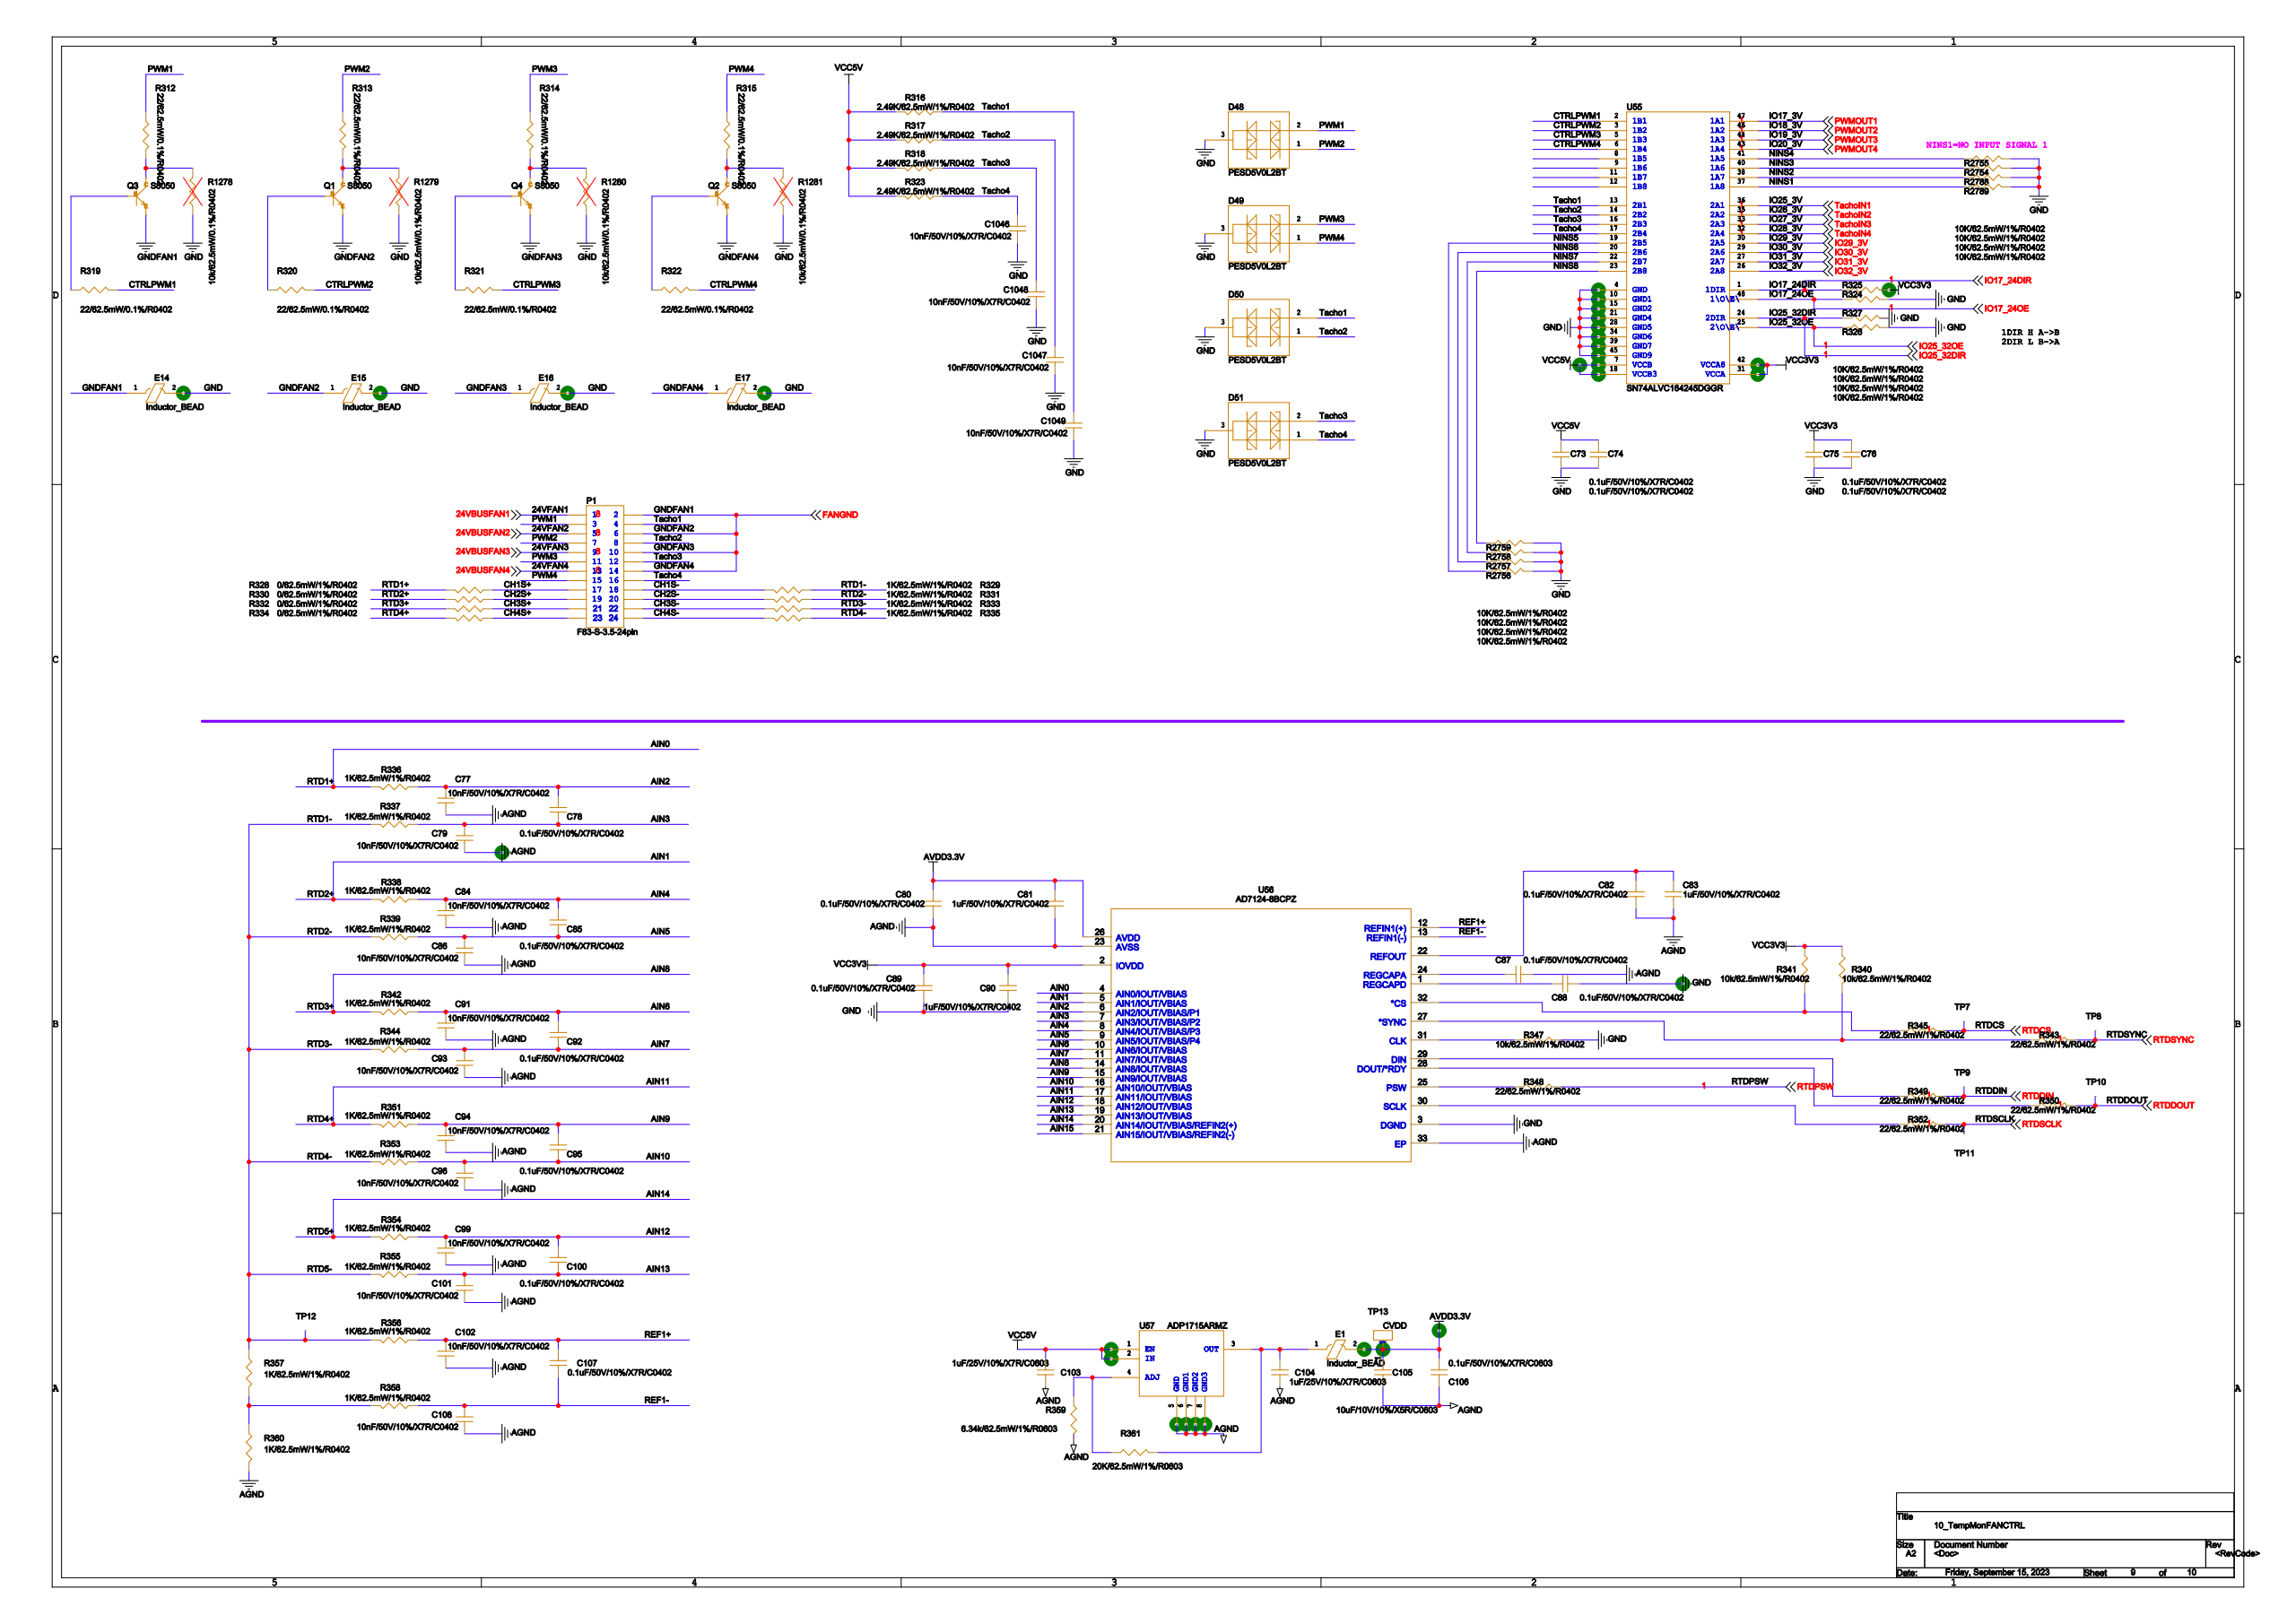Circuit board | Cadence Allegro | 634 parts | 645 nets | one sheet of the schematic
Parts on this sheet (reference | value | footprint):
C73 | 0.1uF/50V/10%/X7R/C0402 | 0402
C74 | 0.1uF/50V/10%/X7R/C0402 | 0402
C75 | 0.1uF/50V/10%/X7R/C0402 | 0402
C76 | 0.1uF/50V/10%/X7R/C0402 | 0402
C77 | 10nF/50V/10%/X7R/C0402 | 0402
C78 | 0.1uF/50V/10%/X7R/C0402 | 0402
C79 | 10nF/50V/10%/X7R/C0402 | 0402
C80 | 0.1uF/50V/10%/X7R/C0402 | 0402
C81 | 1uF/50V/10%/X7R/C0402 | 0402
C82 | 0.1uF/50V/10%/X7R/C0402 | 0402
C83 | 1uF/50V/10%/X7R/C0402 | 0402
C84 | 10nF/50V/10%/X7R/C0402 | 0402
C85 | 0.1uF/50V/10%/X7R/C0402 | 0402
C86 | 10nF/50V/10%/X7R/C0402 | 0402
C87 | 0.1uF/50V/10%/X7R/C0402 | 0402
C88 | 0.1uF/50V/10%/X7R/C0402 | 0402
C89 | 0.1uF/50V/10%/X7R/C0402 | 0402
C90 | 1uF/50V/10%/X7R/C0402 | 0402
C91 | 10nF/50V/10%/X7R/C0402 | 0402
C92 | 0.1uF/50V/10%/X7R/C0402 | 0402
C93 | 10nF/50V/10%/X7R/C0402 | 0402
C94 | 10nF/50V/10%/X7R/C0402 | 0402
C95 | 0.1uF/50V/10%/X7R/C0402 | 0402
C96 | 10nF/50V/10%/X7R/C0402 | 0402
C99 | 10nF/50V/10%/X7R/C0402 | 0402
C100 | 0.1uF/50V/10%/X7R/C0402 | 0402
C101 | 10nF/50V/10%/X7R/C0402 | 0402
C102 | 10nF/50V/10%/X7R/C0402 | 0402
C103 | 1uF/25V/10%/X7R/C0603 | 0603C
C104 | 1uF/25V/10%/X7R/C0603 | 0603C
C105 | 10uF/10V/10%/X5R/C0603 | 0603C
C106 | 0.1uF/50V/10%/X7R/C0603 | 0603C
C107 | 0.1uF/50V/10%/X7R/C0402 | 0402
C108 | 10nF/50V/10%/X7R/C0402 | 0402
C1046 | 10nF/50V/10%/X7R/C0402 | 0402
C1047 | 10nF/50V/10%/X7R/C0402 | 0402
C1048 | 10nF/50V/10%/X7R/C0402 | 0402
C1049 | 10nF/50V/10%/X7R/C0402 | 0402
D48 | PESD5V0L2BT | SOT23
D49 | PESD5V0L2BT | SOT23
D50 | PESD5V0L2BT | SOT23
D51 | PESD5V0L2BT | SOT23
E1 | Inductor_BEAD | 0603R
E14 | Inductor_BEAD | 0603R
E15 | Inductor_BEAD | 0603R
E16 | Inductor_BEAD | 0603R
E17 | Inductor_BEAD | 0603R
P1 | F83-S-3.5-24pin | F83-S-3_5-24PIN
Q1 | S8050 | SOT-23
Q2 | S8050 | SOT-23
Q3 | S8050 | SOT-23
Q4 | S8050 | SOT-23
R312 | 22/62.5mW/0.1%/R0402 | 0402
R313 | 22/62.5mW/0.1%/R0402 | 0402
R314 | 22/62.5mW/0.1%/R0402 | 0402
R315 | 22/62.5mW/0.1%/R0402 | 0402
R316 | 2.49k/62.5mW/1%/R0402 | 0402
R317 | 2.49k/62.5mW/1%/R0402 | 0402
R318 | 2.49k/62.5mW/1%/R0402 | 0402
R319 | 22/62.5mW/0.1%/R0402 | 0402
R320 | 22/62.5mW/0.1%/R0402 | 0402
R321 | 22/62.5mW/0.1%/R0402 | 0402
R322 | 22/62.5mW/0.1%/R0402 | 0402
R323 | 2.49k/62.5mW/1%/R0402 | 0402
R324 | 10K/62.5mW/1%/R0402 | 0402
R325 | 10K/62.5mW/1%/R0402 | 0402
R326 | 10K/62.5mW/1%/R0402 | 0402
R327 | 10K/62.5mW/1%/R0402 | 0402
R328 | 0/62.5mW/1%/R0402 | 0402
R329 | 1K/62.5mW/1%/R0402 | 0402
R330 | 0/62.5mW/1%/R0402 | 0402
R331 | 1K/62.5mW/1%/R0402 | 0402
R332 | 0/62.5mW/1%/R0402 | 0402
R333 | 1K/62.5mW/1%/R0402 | 0402
R334 | 0/62.5mW/1%/R0402 | 0402
R335 | 1K/62.5mW/1%/R0402 | 0402
R336 | 1K/62.5mW/1%/R0402 | 0402
R337 | 1K/62.5mW/1%/R0402 | 0402
R338 | 1K/62.5mW/1%/R0402 | 0402
R339 | 1K/62.5mW/1%/R0402 | 0402
R340 | 10k/62.5mW/1%/R0402 | 0402
R341 | 10k/62.5mW/1%/R0402 | 0402
R342 | 1K/62.5mW/1%/R0402 | 0402
R343 | 22/62.5mW/1%/R0402 | 0402
R344 | 1K/62.5mW/1%/R0402 | 0402
R345 | 22/62.5mW/1%/R0402 | 0402
R347 | 10k/62.5mW/1%/R0402 | 0402
R348 | 22/62.5mW/1%/R0402 | 0402
R349 | 22/62.5mW/1%/R0402 | 0402
R350 | 22/62.5mW/1%/R0402 | 0402
R351 | 1K/62.5mW/1%/R0402 | 0402
R352 | 22/62.5mW/1%/R0402 | 0402
R353 | 1K/62.5mW/1%/R0402 | 0402
R354 | 1K/62.5mW/1%/R0402 | 0402
R355 | 1K/62.5mW/1%/R0402 | 0402
R356 | 1K/62.5mW/1%/R0402 | 0402
R357 | 1K/62.5mW/1%/R0402 | 0402
R358 | 1K/62.5mW/1%/R0402 | 0402
R359 | 6.34k/62.5mW/1%/R0603 | 0603R
R360 | 1K/62.5mW/1%/R0402 | 0402
R361 | 20K/62.5mW/1%/R0603 | 0603R
R1278 | 10k/62.5mW/0.1%/R0402 | 0402
R1279 | 10k/62.5mW/0.1%/R0402 | 0402
R1280 | 10k/62.5mW/0.1%/R0402 | 0402
R1281 | 10k/62.5mW/0.1%/R0402 | 0402
R2754 | 10K/62.5mW/1%/R0402 | 0402
R2755 | 10K/62.5mW/1%/R0402 | 0402
R2756 | 10K/62.5mW/1%/R0402 | 0402
R2757 | 10K/62.5mW/1%/R0402 | 0402
R2758 | 10K/62.5mW/1%/R0402 | 0402
R2759 | 10K/62.5mW/1%/R0402 | 0402
R2788 | 10K/62.5mW/1%/R0402 | 0402
R2789 | 10K/62.5mW/1%/R0402 | 0402
TP7 | TEST POINT A | TEST_12MM
TP8 | TEST POINT A | TEST_12MM
TP9 | TEST POINT A | TEST_12MM
TP10 | TEST POINT A | TEST_12MM
TP11 | TEST POINT A | TEST_12MM
TP12 | TEST POINT A | TEST_12MM
TP13 | CVDD | D0_6
U55 | SN74ALVC164245DGGR | TSSOP-48
U56 | Value | CP_32_12_ADI
U57 | ADP1715ARMZ | MSOP8
Nets of these parts (net: part-pin ...):
AGND: C73-1 C74-1 C75-1 C76-1 C77-2 C79-2 C80-2 C81-2 C82-2 C83-2 C84-2 C86-2 C87-2 C88-2 C89-2 C90-2 C91-2 C93-2 C94-2 C96-2 C99-2 C101-2 C102-2 C103-2 C104-2 C105-2 C106-2 C108-2 C1046-2 C1047-2 C1048-2 C1049-2 D48-3 D49-3 D50-3 D51-3 E14-2 E15-2 E16-2 E17-2 R324-1 R326-1 R327-1 R347-2 R359-1 R360-2 R1278-1 R1279-1 R1280-1 R1281-1 R2754-1 R2755-1 R2756-1 R2757-1 R2758-1 R2759-1 R2788-1 R2789-1 U57-5 U57-6 U57-7 U57-8 U55-4 U55-10 U55-15 U55-21 U55-28 U55-34 U55-39 U55-45 U56-3 U56-23 U56-33
IO25_32DIR: R327-2 U55-24
IO25_32OE: R326-2 U55-25
PWMOUT1: U55-47
3.3V: C75-2 C76-2 C89-1 C90-1 R325-1 R340-1 R341-1 U55-31 U55-42 U56-2
PWMOUT2: U55-46
PWMOUT3: U55-44
PWMOUT4: U55-43
IO17_24DIR: R325-2 U55-1
IO17_24OE: R324-2 U55-48
RTDPSW: R348-2
RTDSYNC: R343-2 TP8-1
RTDDOUT: R350-2 TP10-1
RTDDIN: R349-2 TP9-1
RTDSCLK: R352-2 TP11-1
RTDCS: R345-2 TP7-1
VCC5V: C73-2 C74-2 C103-1 R316-2 R317-2 R318-2 R323-2 U57-1 U57-2 U55-7 U55-18
N23420107: Q3-3 R312-2 R1278-2
N23420396: Q1-3 R313-2 R1279-2
N23420476: Q4-3 R314-2 R1280-2
N23420600: Q2-3 R315-2 R1281-2
TACHO1: C1049-1 D50-2 R316-1 P1-4 U55-13
TACHO2: C1047-1 D50-1 R317-1 P1-8 U55-14
TACHO3: C1048-1 D51-2 R318-1 P1-12 U55-16
TACHO4: C1046-1 D51-1 R323-1 P1-16 U55-17
24VBUSFAN1: P1-1
24VBUSFAN2: P1-5
24VBUSFAN3: P1-9
24VBUSFAN4: P1-13
PWM1: D48-2 R312-1 P1-3
PWM2: D48-1 R313-1 P1-7
PWM3: D49-2 R314-1 P1-11
PWM4: D49-1 R315-1 P1-15
N23420104: Q3-1 R319-1
CTRLPWM1: R319-2 U55-2
N23420393: Q1-1 R320-1
CTRLPWM2: R320-2 U55-3
N23420473: Q4-1 R321-1
CTRLPWM3: R321-2 U55-5
N23420597: Q2-1 R322-1
CTRLPWM4: R322-2 U55-6
AVDD3.3V: C80-1 C81-1 C105-1 C106-1 E1-2 TP13-1 U56-26
N23528814: C104-1 E1-1 R361-1 U57-3
N23528786: R359-2 R361-2 U57-4
FANGND: E14-1 E15-1 E16-1 E17-1 Q1-2 Q2-2 Q3-2 Q4-2 P1-2 P1-6 P1-10 P1-14
CH1S+: R328-1 P1-17
CH1S-: R329-2 P1-18
CH2S+: R330-1 P1-19
CH2S-: R331-2 P1-20
CH3S+: R332-1 P1-21
CH3S-: R333-2 P1-22
CH4S+: R334-1 P1-23
CH4S-: R335-2 P1-24
AIN12: C99-1 C100-1 R354-1 U56-18
AIN13: C100-2 C101-1 R355-1 U56-19
REF1+: C102-1 C107-1 R356-1 U56-12
REF1-: C107-2 C108-1 R358-1 U56-13
N23186180: C87-1 U56-24
AIN6: C91-1 C92-1 R342-1 U56-10
AIN7: C92-2 C93-1 R344-1 U56-11
AIN2: C77-1 C78-1 R336-1 U56-6
AIN3: C78-2 C79-1 R337-1 U56-7
N23186471: C82-1 C83-1 U56-22
AIN4: C84-1 C85-1 R338-1 U56-8
AIN5: C85-2 C86-1 R339-1 U56-9
N23186182: C88-1 U56-1
AIN9: C94-1 C95-1 R351-1 U56-15
AIN10: C95-2 C96-1 R353-1 U56-16
RTD1-: R329-1 R331-1 R333-1 R335-1 R337-2 R339-2 R344-2 R353-2 R355-2 R356-2 R357-1 TP12-1
AIN0: R328-2 R336-2 U56-4
AIN1: R330-2 R338-2 U56-5
AIN8: R332-2 R342-2 U56-14
AIN11: R334-2 R351-2 U56-17
AIN14: R354-2 U56-20
N23184433: R357-2 R358-2 R360-1
NINS3: R2754-2 U55-40
NINS4: R2755-2 U55-41
NINS5: R2756-2 U55-19
NINS6: R2757-2 U55-20
NINS7: R2758-2 U55-22
NINS8: R2759-2 U55-23
NINS2: R2788-2 U55-38
NINS1: R2789-2 U55-37
N23186325: R340-2 R343-1 U56-27
N23186319: R341-2 R345-1 U56-32
N23186239: R347-1 U56-31
N23186243: R348-1 U56-25
N23186381: R349-1 U56-29
N23186383: R350-1 U56-28
N23186389: R352-1 U56-30
IO29_3V: U55-30
IO30_3V: U55-29
IO31_3V: U55-27
IO32_3V: U55-26
AIN15: U56-21